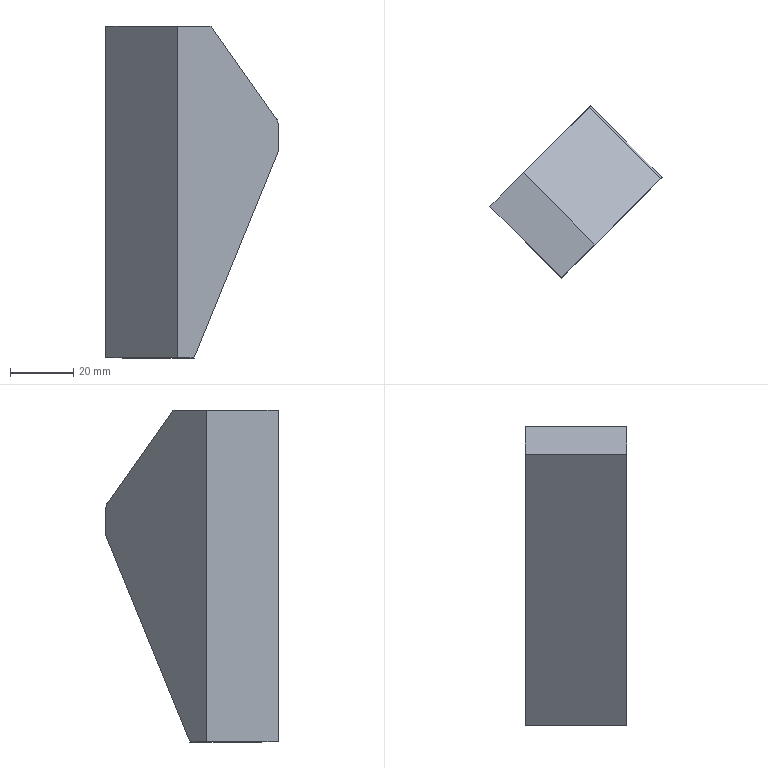Part | NX | features solid 2 | 1 solid | 10 faces | box 54.447 x 54.447 x 105 mm | volume 97768 mm3 | plane 8 | cylinder 2 | commonest cylinder face diameters 4 x2
STEP:
#1=CARTESIAN_POINT('',(-851.357,-661.852,-90.));
#2=VERTEX_POINT('',#1);
#3=CARTESIAN_POINT('',(-846.073,-656.568,-90.));
#4=VERTEX_POINT('',#3);
#5=CARTESIAN_POINT('',(-851.357,-661.852,-90.));
#6=DIRECTION('',(0.7071,0.7071,0.));
#7=VECTOR('',#6,1000.);
#8=LINE('',#5,#7);
#9=EDGE_CURVE('',#2,#4,#8,.T.);
#10=ORIENTED_EDGE('',*,*,#9,.F.);
#11=CARTESIAN_POINT('',(-873.984,-639.225,-90.));
#12=VERTEX_POINT('',#11);
#13=CARTESIAN_POINT('',(-873.984,-639.225,-90.));
#14=DIRECTION('',(0.7071,-0.7071,0.));
#15=VECTOR('',#14,1000.);
#16=LINE('',#13,#15);
#17=EDGE_CURVE('',#12,#2,#16,.T.);
#18=ORIENTED_EDGE('',*,*,#17,.F.);
#19=CARTESIAN_POINT('',(-868.7,-633.941,-90.));
#20=VERTEX_POINT('',#19);
#21=CARTESIAN_POINT('',(-873.984,-639.225,-90.));
#22=DIRECTION('',(0.7071,0.7071,0.));
#23=VECTOR('',#22,1000.);
#24=LINE('',#21,#23);
#25=EDGE_CURVE('',#12,#20,#24,.T.);
#26=ORIENTED_EDGE('',*,*,#25,.T.);
#27=CARTESIAN_POINT('',(-868.7,-633.941,-90.));
#28=DIRECTION('',(0.7071,-0.7071,0.));
#29=VECTOR('',#28,1000.);
#30=LINE('',#27,#29);
#31=EDGE_CURVE('',#20,#4,#30,.T.);
#32=ORIENTED_EDGE('',*,*,#31,.T.);
#33=EDGE_LOOP('',(#10,#18,#26,#32));
#34=FACE_BOUND('',#33,.T.);
#35=CARTESIAN_POINT('',(-873.984,-639.225,-90.));
#36=DIRECTION('',(0.,0.,-1.));
#37=DIRECTION('',(-0.7071,-0.7071,0.));
#38=AXIS2_PLACEMENT_3D('',#35,#36,#37);
#39=PLANE('',#38);
#40=ADVANCED_FACE('',(#34),#39,.T.);
#41=CARTESIAN_POINT('',(-819.726,-630.222,-25.464));
#42=VERTEX_POINT('',#41);
#43=CARTESIAN_POINT('',(-846.073,-656.568,-90.));
#44=DIRECTION('',(0.3536,0.3536,0.866));
#45=VECTOR('',#44,1000.);
#46=LINE('',#43,#45);
#47=EDGE_CURVE('',#4,#42,#46,.T.);
#48=ORIENTED_EDGE('',*,*,#47,.F.);
#49=ORIENTED_EDGE('',*,*,#31,.F.);
#50=CARTESIAN_POINT('',(-842.354,-607.594,-25.464));
#51=VERTEX_POINT('',#50);
#52=CARTESIAN_POINT('',(-868.7,-633.941,-90.));
#53=DIRECTION('',(0.3536,0.3536,0.866));
#54=VECTOR('',#53,1000.);
#55=LINE('',#52,#54);
#56=EDGE_CURVE('',#20,#51,#55,.T.);
#57=ORIENTED_EDGE('',*,*,#56,.T.);
#58=CARTESIAN_POINT('',(-842.354,-607.594,-25.464));
#59=DIRECTION('',(0.7071,-0.7071,0.));
#60=VECTOR('',#59,1000.);
#61=LINE('',#58,#60);
#62=EDGE_CURVE('',#51,#42,#61,.T.);
#63=ORIENTED_EDGE('',*,*,#62,.T.);
#64=EDGE_LOOP('',(#48,#49,#57,#63));
#65=FACE_BOUND('',#64,.T.);
#66=CARTESIAN_POINT('',(-868.7,-633.941,-90.));
#67=DIRECTION('',(0.6124,0.6124,-0.5));
#68=DIRECTION('',(-0.3536,-0.3536,-0.866));
#69=AXIS2_PLACEMENT_3D('',#66,#67,#68);
#70=PLANE('',#69);
#71=ADVANCED_FACE('',(#65),#70,.T.);
#72=CARTESIAN_POINT('',(-819.537,-630.032,-24.464));
#73=VERTEX_POINT('',#72);
#74=CARTESIAN_POINT('',(-820.951,-631.446,-24.464));
#75=DIRECTION('',(-0.7071,0.7071,0.));
#76=DIRECTION('',(-0.7071,-0.7071,0.));
#77=AXIS2_PLACEMENT_3D('',#74,#75,#76);
#78=CIRCLE('',#77,2.);
#79=EDGE_CURVE('',#73,#42,#78,.T.);
#80=ORIENTED_EDGE('',*,*,#79,.T.);
#81=ORIENTED_EDGE('',*,*,#62,.F.);
#82=CARTESIAN_POINT('',(-842.164,-607.405,-24.464));
#83=VERTEX_POINT('',#82);
#84=CARTESIAN_POINT('',(-843.578,-608.819,-24.464));
#85=DIRECTION('',(-0.7071,0.7071,0.));
#86=DIRECTION('',(-0.7071,-0.7071,0.));
#87=AXIS2_PLACEMENT_3D('',#84,#85,#86);
#88=CIRCLE('',#87,2.);
#89=EDGE_CURVE('',#83,#51,#88,.T.);
#90=ORIENTED_EDGE('',*,*,#89,.F.);
#91=CARTESIAN_POINT('',(-842.164,-607.405,-24.464));
#92=DIRECTION('',(0.7071,-0.7071,0.));
#93=VECTOR('',#92,1000.);
#94=LINE('',#91,#93);
#95=EDGE_CURVE('',#83,#73,#94,.T.);
#96=ORIENTED_EDGE('',*,*,#95,.T.);
#97=EDGE_LOOP('',(#80,#81,#90,#96));
#98=FACE_BOUND('',#97,.T.);
#99=CARTESIAN_POINT('',(-843.578,-608.819,-24.464));
#100=DIRECTION('',(0.7071,-0.7071,0.));
#101=DIRECTION('',(0.,0.,-1.));
#102=AXIS2_PLACEMENT_3D('',#99,#100,#101);
#103=CYLINDRICAL_SURFACE('',#102,2.);
#104=ADVANCED_FACE('',(#98),#103,.T.);
#105=CARTESIAN_POINT('',(-819.537,-630.032,-15.828));
#106=VERTEX_POINT('',#105);
#107=CARTESIAN_POINT('',(-819.537,-630.032,-24.464));
#108=DIRECTION('',(0.,0.,1.));
#109=VECTOR('',#108,1000.);
#110=LINE('',#107,#109);
#111=EDGE_CURVE('',#73,#106,#110,.T.);
#112=ORIENTED_EDGE('',*,*,#111,.F.);
#113=ORIENTED_EDGE('',*,*,#95,.F.);
#114=CARTESIAN_POINT('',(-842.164,-607.405,-15.828));
#115=VERTEX_POINT('',#114);
#116=CARTESIAN_POINT('',(-842.164,-607.405,-24.464));
#117=DIRECTION('',(0.,0.,1.));
#118=VECTOR('',#117,1000.);
#119=LINE('',#116,#118);
#120=EDGE_CURVE('',#83,#115,#119,.T.);
#121=ORIENTED_EDGE('',*,*,#120,.T.);
#122=CARTESIAN_POINT('',(-842.164,-607.405,-15.828));
#123=DIRECTION('',(0.7071,-0.7071,0.));
#124=VECTOR('',#123,1000.);
#125=LINE('',#122,#124);
#126=EDGE_CURVE('',#115,#106,#125,.T.);
#127=ORIENTED_EDGE('',*,*,#126,.T.);
#128=EDGE_LOOP('',(#112,#113,#121,#127));
#129=FACE_BOUND('',#128,.T.);
#130=CARTESIAN_POINT('',(-842.164,-607.405,-24.464));
#131=DIRECTION('',(0.7071,0.7071,0.));
#132=DIRECTION('',(0.,0.,-1.));
#133=AXIS2_PLACEMENT_3D('',#130,#131,#132);
#134=PLANE('',#133);
#135=ADVANCED_FACE('',(#129),#134,.T.);
#136=CARTESIAN_POINT('',(-819.951,-630.446,-14.414));
#137=VERTEX_POINT('',#136);
#138=CARTESIAN_POINT('',(-820.951,-631.446,-15.828));
#139=DIRECTION('',(-0.7071,0.7071,0.));
#140=DIRECTION('',(-0.7071,-0.7071,0.));
#141=AXIS2_PLACEMENT_3D('',#138,#139,#140);
#142=CIRCLE('',#141,2.);
#143=EDGE_CURVE('',#137,#106,#142,.T.);
#144=ORIENTED_EDGE('',*,*,#143,.T.);
#145=ORIENTED_EDGE('',*,*,#126,.F.);
#146=CARTESIAN_POINT('',(-842.578,-607.819,-14.414));
#147=VERTEX_POINT('',#146);
#148=CARTESIAN_POINT('',(-843.578,-608.819,-15.828));
#149=DIRECTION('',(-0.7071,0.7071,0.));
#150=DIRECTION('',(-0.7071,-0.7071,0.));
#151=AXIS2_PLACEMENT_3D('',#148,#149,#150);
#152=CIRCLE('',#151,2.);
#153=EDGE_CURVE('',#147,#115,#152,.T.);
#154=ORIENTED_EDGE('',*,*,#153,.F.);
#155=CARTESIAN_POINT('',(-842.578,-607.819,-14.414));
#156=DIRECTION('',(0.7071,-0.7071,0.));
#157=VECTOR('',#156,1000.);
#158=LINE('',#155,#157);
#159=EDGE_CURVE('',#147,#137,#158,.T.);
#160=ORIENTED_EDGE('',*,*,#159,.T.);
#161=EDGE_LOOP('',(#144,#145,#154,#160));
#162=FACE_BOUND('',#161,.T.);
#163=CARTESIAN_POINT('',(-843.578,-608.819,-15.828));
#164=DIRECTION('',(0.7071,-0.7071,0.));
#165=DIRECTION('',(0.,0.,-1.));
#166=AXIS2_PLACEMENT_3D('',#163,#164,#165);
#167=CYLINDRICAL_SURFACE('',#166,2.);
#168=ADVANCED_FACE('',(#162),#167,.T.);
#169=CARTESIAN_POINT('',(-840.75,-651.245,15.));
#170=VERTEX_POINT('',#169);
#171=CARTESIAN_POINT('',(-819.951,-630.446,-14.414));
#172=DIRECTION('',(-0.5,-0.5,0.7071));
#173=VECTOR('',#172,1000.);
#174=LINE('',#171,#173);
#175=EDGE_CURVE('',#137,#170,#174,.T.);
#176=ORIENTED_EDGE('',*,*,#175,.F.);
#177=ORIENTED_EDGE('',*,*,#159,.F.);
#178=CARTESIAN_POINT('',(-863.377,-628.618,15.));
#179=VERTEX_POINT('',#178);
#180=CARTESIAN_POINT('',(-842.578,-607.819,-14.414));
#181=DIRECTION('',(-0.5,-0.5,0.7071));
#182=VECTOR('',#181,1000.);
#183=LINE('',#180,#182);
#184=EDGE_CURVE('',#147,#179,#183,.T.);
#185=ORIENTED_EDGE('',*,*,#184,.T.);
#186=CARTESIAN_POINT('',(-863.377,-628.618,15.));
#187=DIRECTION('',(0.7071,-0.7071,0.));
#188=VECTOR('',#187,1000.);
#189=LINE('',#186,#188);
#190=EDGE_CURVE('',#179,#170,#189,.T.);
#191=ORIENTED_EDGE('',*,*,#190,.T.);
#192=EDGE_LOOP('',(#176,#177,#185,#191));
#193=FACE_BOUND('',#192,.T.);
#194=CARTESIAN_POINT('',(-842.578,-607.819,-14.414));
#195=DIRECTION('',(0.5,0.5,0.7071));
#196=DIRECTION('',(0.5,0.5,-0.7071));
#197=AXIS2_PLACEMENT_3D('',#194,#195,#196);
#198=PLANE('',#197);
#199=ADVANCED_FACE('',(#193),#198,.T.);
#200=CARTESIAN_POINT('',(-851.357,-661.852,15.));
#201=VERTEX_POINT('',#200);
#202=CARTESIAN_POINT('',(-840.75,-651.245,15.));
#203=DIRECTION('',(-0.7071,-0.7071,0.));
#204=VECTOR('',#203,1000.);
#205=LINE('',#202,#204);
#206=EDGE_CURVE('',#170,#201,#205,.T.);
#207=ORIENTED_EDGE('',*,*,#206,.F.);
#208=ORIENTED_EDGE('',*,*,#190,.F.);
#209=CARTESIAN_POINT('',(-873.984,-639.225,15.));
#210=VERTEX_POINT('',#209);
#211=CARTESIAN_POINT('',(-863.377,-628.618,15.));
#212=DIRECTION('',(-0.7071,-0.7071,0.));
#213=VECTOR('',#212,1000.);
#214=LINE('',#211,#213);
#215=EDGE_CURVE('',#179,#210,#214,.T.);
#216=ORIENTED_EDGE('',*,*,#215,.T.);
#217=CARTESIAN_POINT('',(-873.984,-639.225,15.));
#218=DIRECTION('',(0.7071,-0.7071,0.));
#219=VECTOR('',#218,1000.);
#220=LINE('',#217,#219);
#221=EDGE_CURVE('',#210,#201,#220,.T.);
#222=ORIENTED_EDGE('',*,*,#221,.T.);
#223=EDGE_LOOP('',(#207,#208,#216,#222));
#224=FACE_BOUND('',#223,.T.);
#225=CARTESIAN_POINT('',(-863.377,-628.618,15.));
#226=DIRECTION('',(0.,0.,1.));
#227=DIRECTION('',(0.7071,0.7071,0.));
#228=AXIS2_PLACEMENT_3D('',#225,#226,#227);
#229=PLANE('',#228);
#230=ADVANCED_FACE('',(#224),#229,.T.);
#231=CARTESIAN_POINT('',(-851.357,-661.852,15.));
#232=DIRECTION('',(0.,0.,-1.));
#233=VECTOR('',#232,1000.);
#234=LINE('',#231,#233);
#235=EDGE_CURVE('',#201,#2,#234,.T.);
#236=ORIENTED_EDGE('',*,*,#235,.F.);
#237=ORIENTED_EDGE('',*,*,#221,.F.);
#238=CARTESIAN_POINT('',(-873.984,-639.225,15.));
#239=DIRECTION('',(0.,0.,-1.));
#240=VECTOR('',#239,1000.);
#241=LINE('',#238,#240);
#242=EDGE_CURVE('',#210,#12,#241,.T.);
#243=ORIENTED_EDGE('',*,*,#242,.T.);
#244=ORIENTED_EDGE('',*,*,#17,.T.);
#245=EDGE_LOOP('',(#236,#237,#243,#244));
#246=FACE_BOUND('',#245,.T.);
#247=CARTESIAN_POINT('',(-873.984,-639.225,15.));
#248=DIRECTION('',(-0.7071,-0.7071,0.));
#249=DIRECTION('',(0.,0.,1.));
#250=AXIS2_PLACEMENT_3D('',#247,#248,#249);
#251=PLANE('',#250);
#252=ADVANCED_FACE('',(#246),#251,.T.);
#253=ORIENTED_EDGE('',*,*,#25,.F.);
#254=ORIENTED_EDGE('',*,*,#242,.F.);
#255=ORIENTED_EDGE('',*,*,#215,.F.);
#256=ORIENTED_EDGE('',*,*,#184,.F.);
#257=ORIENTED_EDGE('',*,*,#153,.T.);
#258=ORIENTED_EDGE('',*,*,#120,.F.);
#259=ORIENTED_EDGE('',*,*,#89,.T.);
#260=ORIENTED_EDGE('',*,*,#56,.F.);
#261=EDGE_LOOP('',(#253,#254,#255,#256,#257,#258,#259,#260));
#262=FACE_BOUND('',#261,.T.);
#263=CARTESIAN_POINT('',(-843.578,-608.819,-24.464));
#264=DIRECTION('',(-0.7071,0.7071,0.));
#265=DIRECTION('',(0.,0.,1.));
#266=AXIS2_PLACEMENT_3D('',#263,#264,#265);
#267=PLANE('',#266);
#268=ADVANCED_FACE('',(#262),#267,.T.);
#269=ORIENTED_EDGE('',*,*,#9,.T.);
#270=ORIENTED_EDGE('',*,*,#47,.T.);
#271=ORIENTED_EDGE('',*,*,#79,.F.);
#272=ORIENTED_EDGE('',*,*,#111,.T.);
#273=ORIENTED_EDGE('',*,*,#143,.F.);
#274=ORIENTED_EDGE('',*,*,#175,.T.);
#275=ORIENTED_EDGE('',*,*,#206,.T.);
#276=ORIENTED_EDGE('',*,*,#235,.T.);
#277=EDGE_LOOP('',(#269,#270,#271,#272,#273,#274,#275,#276));
#278=FACE_BOUND('',#277,.T.);
#279=CARTESIAN_POINT('',(-820.951,-631.446,-24.464));
#280=DIRECTION('',(-0.7071,0.7071,0.));
#281=DIRECTION('',(0.,0.,1.));
#282=AXIS2_PLACEMENT_3D('',#279,#280,#281);
#283=PLANE('',#282);
#284=ADVANCED_FACE('',(#278),#283,.F.);
#285=CLOSED_SHELL('',(#40,#71,#104,#135,#168,#199,#230,#252,#268,#284));
#286=MANIFOLD_SOLID_BREP('',#285);
#287=(LENGTH_UNIT()NAMED_UNIT(*)SI_UNIT(.MILLI.,.METRE.));
#288=UNCERTAINTY_MEASURE_WITH_UNIT(LENGTH_MEASURE(0.00001),#287,'','');
#289=(NAMED_UNIT(*)PLANE_ANGLE_UNIT()SI_UNIT($,.RADIAN.));
#290=(NAMED_UNIT(*)SI_UNIT($,.STERADIAN.)SOLID_ANGLE_UNIT());
#291=(GEOMETRIC_REPRESENTATION_CONTEXT(3)GLOBAL_UNCERTAINTY_ASSIGNED_CONTEXT((#288))GLOBAL_UNIT_ASSIGNED_CONTEXT((#287,#289,#290))REPRESENTATION_CONTEXT('',''));
#292=ADVANCED_BREP_SHAPE_REPRESENTATION('',(#286),#291);